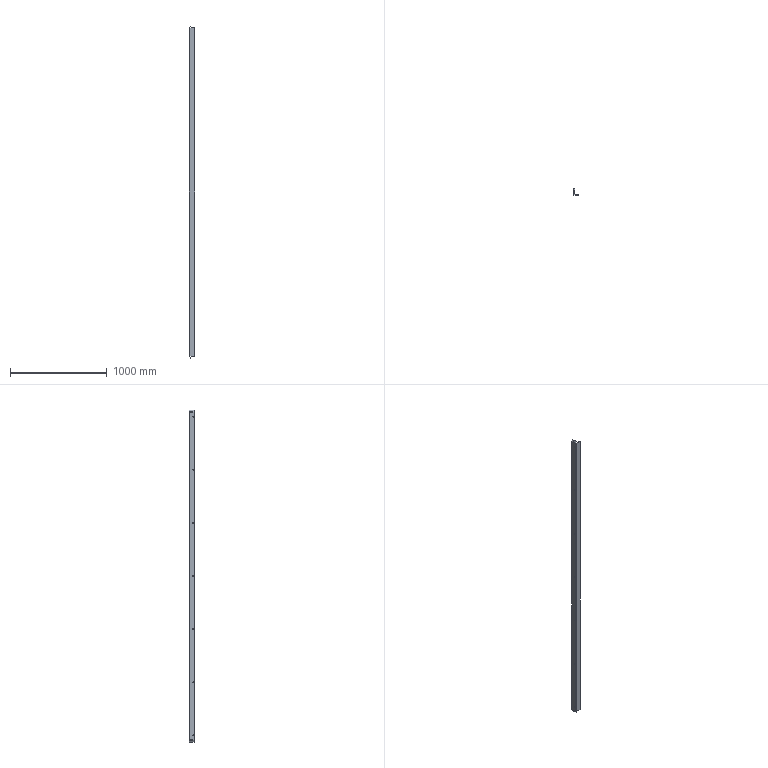Part | STEP file | BCC3 H11_1B | 1 solid | 46 faces | box 60 x 60 x 3440 mm | volume 1915667 mm3 | plane 26 | cylinder 20 | commonest cylinder face diameters 10 x14 8 x3 18 x3